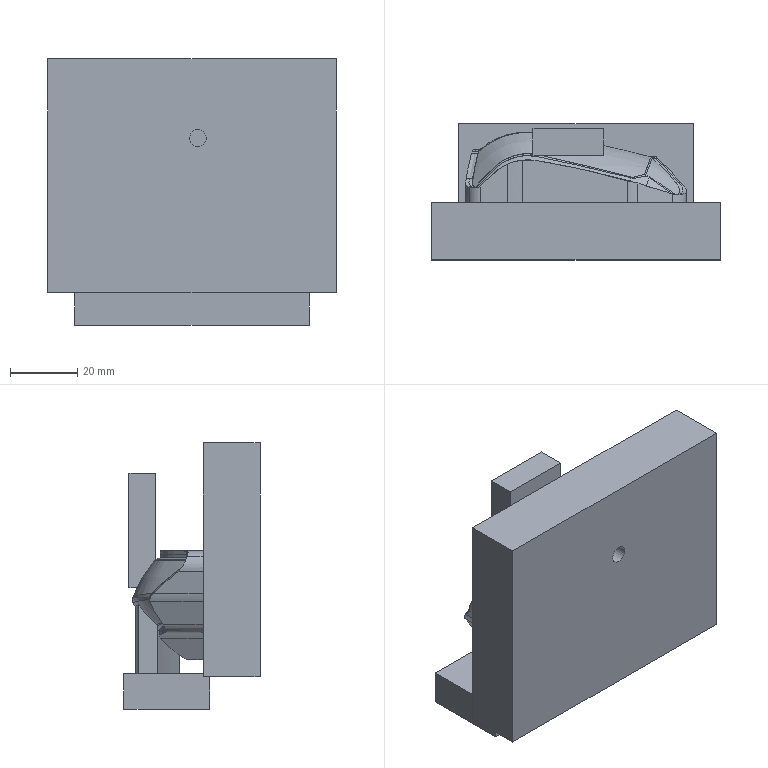Part | 6 solids | 1287 faces | box 85.5 x 40.385 x 79 mm | volume 142105 mm3 | spline 858 | cylinder 252 | plane 96 | sphere 37 | torus 35 | cone 9 | commonest cylinder face diameters 1 x34 0.2 x22 2 x15 1.9 x13 1.2 x12 1.4 x10